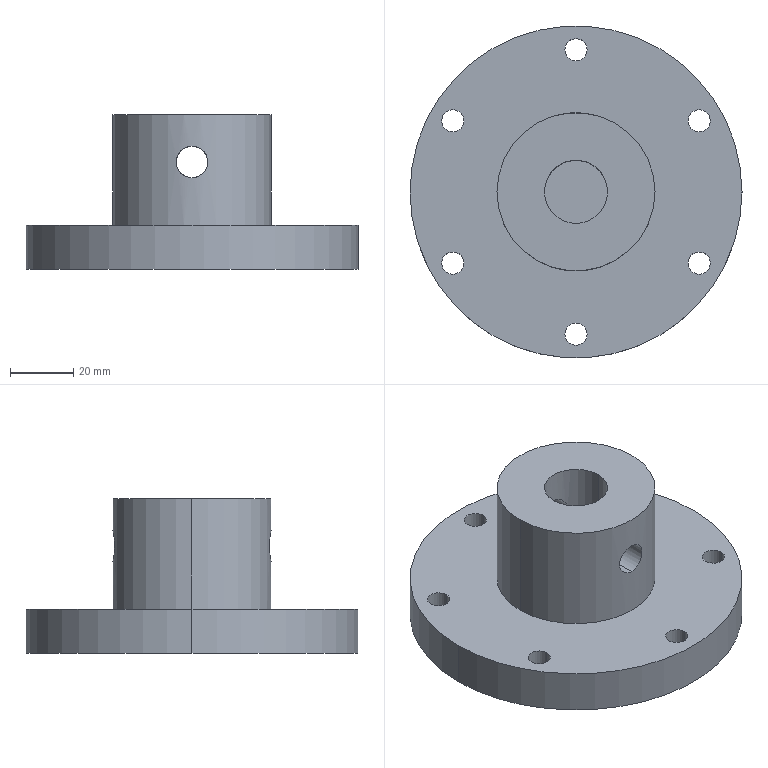Part | SolidWorks | features ICE 2, Extrusion 1 | 1 solid | 26 faces | box 105 x 105 x 49 mm | volume 173332 mm3 | cylinder 22 | plane 4 | commonest cylinder face diameters 7 x12 10 x4 20 x2 50 x2 105 x2
STEP:
#1=CARTESIAN_POINT('',(0.,-25.,29.));
#2=VERTEX_POINT('',#1);
#3=CARTESIAN_POINT('',(0.,-25.,39.));
#4=VERTEX_POINT('',#3);
#5=CARTESIAN_POINT('',(0.,-25.,29.));
#6=CARTESIAN_POINT('',(-0.3267,-25.,29.));
#7=CARTESIAN_POINT('',(-0.652,-24.994,29.032));
#8=CARTESIAN_POINT('',(-1.3,-24.968,29.161));
#9=CARTESIAN_POINT('',(-1.614,-24.95,29.256));
#10=CARTESIAN_POINT('',(-2.065,-24.915,29.444));
#11=CARTESIAN_POINT('',(-2.213,-24.902,29.513));
#12=CARTESIAN_POINT('',(-2.502,-24.875,29.668));
#13=CARTESIAN_POINT('',(-2.644,-24.86,29.753));
#14=CARTESIAN_POINT('',(-3.052,-24.815,30.026));
#15=CARTESIAN_POINT('',(-3.303,-24.782,30.232));
#16=CARTESIAN_POINT('',(-3.764,-24.716,30.693));
#17=CARTESIAN_POINT('',(-3.975,-24.683,30.949));
#18=CARTESIAN_POINT('',(-4.337,-24.622,31.49));
#19=CARTESIAN_POINT('',(-4.491,-24.594,31.777));
#20=CARTESIAN_POINT('',(-4.743,-24.546,32.384));
#21=CARTESIAN_POINT('',(-4.839,-24.527,32.7));
#22=CARTESIAN_POINT('',(-4.967,-24.502,33.34));
#23=CARTESIAN_POINT('',(-5.,-24.495,33.667));
#24=CARTESIAN_POINT('',(-5.,-24.495,34.328));
#25=CARTESIAN_POINT('',(-4.968,-24.502,34.653));
#26=CARTESIAN_POINT('',(-4.841,-24.527,35.294));
#27=CARTESIAN_POINT('',(-4.744,-24.546,35.612));
#28=CARTESIAN_POINT('',(-4.494,-24.593,36.216));
#29=CARTESIAN_POINT('',(-4.341,-24.621,36.503));
#30=CARTESIAN_POINT('',(-4.068,-24.667,36.912));
#31=CARTESIAN_POINT('',(-3.97,-24.683,37.045));
#32=CARTESIAN_POINT('',(-3.762,-24.716,37.298));
#33=CARTESIAN_POINT('',(-3.653,-24.732,37.418));
#34=CARTESIAN_POINT('',(-3.308,-24.781,37.763));
#35=CARTESIAN_POINT('',(-3.057,-24.814,37.971));
#36=CARTESIAN_POINT('',(-2.509,-24.875,38.337));
#37=CARTESIAN_POINT('',(-2.222,-24.903,38.491));
#38=CARTESIAN_POINT('',(-1.62,-24.949,38.741));
#39=CARTESIAN_POINT('',(-1.303,-24.968,38.838));
#40=CARTESIAN_POINT('',(-0.658,-24.993,38.967));
#41=CARTESIAN_POINT('',(-0.3312,-25.,39.));
#42=CARTESIAN_POINT('',(0.,-25.,39.));
#43=B_SPLINE_CURVE_WITH_KNOTS('',3,(#5,#6,#7,#8,#9,#10,#11,#12,#13,#14,#15,#16,#17,#18,#19,#20,#21,#22,#23,#24,#25,#26,#27,#28,#29,#30,#31,#32,#33,#34,#35,#36,#37,#38,#39,#40,#41,#42),.UNSPECIFIED.,.F.,.F.,(4,2,2,2,2,2,2,2,2,2,2,2,2,2,2,2,2,2,4),(0.01567,0.01665,0.01763,0.01812,0.01861,0.01959,0.02057,0.02155,0.02253,0.02351,0.02449,0.02546,0.02644,0.02693,0.02742,0.0284,0.02938,0.03036,0.03134),.UNSPECIFIED.);
#44=EDGE_CURVE('',#2,#4,#43,.T.);
#45=ORIENTED_EDGE('',*,*,#44,.F.);
#46=CARTESIAN_POINT('',(0.,-10.,29.));
#47=VERTEX_POINT('',#46);
#48=CARTESIAN_POINT('',(0.,-52.5,29.));
#49=DIRECTION('',(0.,1.,0.));
#50=VECTOR('',#49,1000.);
#51=LINE('',#48,#50);
#52=EDGE_CURVE('',#2,#47,#51,.T.);
#53=ORIENTED_EDGE('',*,*,#52,.T.);
#54=CARTESIAN_POINT('',(0.,-10.,39.));
#55=VERTEX_POINT('',#54);
#56=CARTESIAN_POINT('',(0.,-10.,29.));
#57=CARTESIAN_POINT('',(-0.3314,-10.,29.));
#58=CARTESIAN_POINT('',(-0.6687,-9.983,29.034));
#59=CARTESIAN_POINT('',(-1.317,-9.918,29.165));
#60=CARTESIAN_POINT('',(-1.631,-9.871,29.262));
#61=CARTESIAN_POINT('',(-2.24,-9.751,29.518));
#62=CARTESIAN_POINT('',(-2.526,-9.68,29.673));
#63=CARTESIAN_POINT('',(-3.061,-9.524,30.034));
#64=CARTESIAN_POINT('',(-3.314,-9.438,30.242));
#65=CARTESIAN_POINT('',(-3.767,-9.266,30.697));
#66=CARTESIAN_POINT('',(-3.971,-9.18,30.944));
#67=CARTESIAN_POINT('',(-4.331,-9.016,31.48));
#68=CARTESIAN_POINT('',(-4.487,-8.938,31.769));
#69=CARTESIAN_POINT('',(-4.737,-8.808,32.367));
#70=CARTESIAN_POINT('',(-4.834,-8.754,32.679));
#71=CARTESIAN_POINT('',(-4.933,-8.699,33.168));
#72=CARTESIAN_POINT('',(-4.958,-8.684,33.334));
#73=CARTESIAN_POINT('',(-4.991,-8.665,33.664));
#74=CARTESIAN_POINT('',(-5.008,-8.656,33.994));
#75=CARTESIAN_POINT('',(-4.992,-8.665,34.325));
#76=CARTESIAN_POINT('',(-4.959,-8.684,34.657));
#77=CARTESIAN_POINT('',(-4.935,-8.698,34.823));
#78=CARTESIAN_POINT('',(-4.836,-8.753,35.311));
#79=CARTESIAN_POINT('',(-4.74,-8.806,35.625));
#80=CARTESIAN_POINT('',(-4.487,-8.938,36.23));
#81=CARTESIAN_POINT('',(-4.332,-9.015,36.518));
#82=CARTESIAN_POINT('',(-3.973,-9.179,37.053));
#83=CARTESIAN_POINT('',(-3.767,-9.267,37.304));
#84=CARTESIAN_POINT('',(-3.311,-9.439,37.761));
#85=CARTESIAN_POINT('',(-3.064,-9.523,37.965));
#86=CARTESIAN_POINT('',(-2.528,-9.679,38.326));
#87=CARTESIAN_POINT('',(-2.237,-9.751,38.483));
#88=CARTESIAN_POINT('',(-1.635,-9.87,38.736));
#89=CARTESIAN_POINT('',(-1.323,-9.918,38.833));
#90=CARTESIAN_POINT('',(-0.6735,-9.983,38.965));
#91=CARTESIAN_POINT('',(-0.3359,-10.,39.));
#92=CARTESIAN_POINT('',(0.,-10.,39.));
#93=B_SPLINE_CURVE_WITH_KNOTS('',3,(#56,#57,#58,#59,#60,#61,#62,#63,#64,#65,#66,#67,#68,#69,#70,#71,#72,#73,#74,#75,#76,#77,#78,#79,#80,#81,#82,#83,#84,#85,#86,#87,#88,#89,#90,#91,#92),.UNSPECIFIED.,.F.,.F.,(4,2,2,2,2,2,2,2,2,1,2,2,2,2,2,2,2,2,4),(0.0159,0.0169,0.01789,0.01888,0.01987,0.02087,0.02186,0.02285,0.02335,0.02384,0.02434,0.02484,0.02583,0.02682,0.02781,0.02881,0.0298,0.03079,0.03178),.UNSPECIFIED.);
#94=EDGE_CURVE('',#47,#55,#93,.T.);
#95=ORIENTED_EDGE('',*,*,#94,.T.);
#96=CARTESIAN_POINT('',(0.,-52.5,39.));
#97=DIRECTION('',(0.,1.,0.));
#98=VECTOR('',#97,1000.);
#99=LINE('',#96,#98);
#100=EDGE_CURVE('',#4,#55,#99,.T.);
#101=ORIENTED_EDGE('',*,*,#100,.F.);
#102=EDGE_LOOP('',(#45,#53,#95,#101));
#103=FACE_OUTER_BOUND('',#102,.T.);
#104=CARTESIAN_POINT('',(0.,-52.5,34.));
#105=DIRECTION('',(0.,1.,0.));
#106=DIRECTION('',(0.,0.,1.));
#107=AXIS2_PLACEMENT_3D('',#104,#105,#106);
#108=CYLINDRICAL_SURFACE('',#107,5.);
#109=ADVANCED_FACE('',(#103),#108,.F.);
#110=CARTESIAN_POINT('',(0.,10.,39.));
#111=VERTEX_POINT('',#110);
#112=CARTESIAN_POINT('',(0.,10.,29.));
#113=VERTEX_POINT('',#112);
#114=CARTESIAN_POINT('',(0.,10.,39.));
#115=CARTESIAN_POINT('',(-0.3365,10.,39.));
#116=CARTESIAN_POINT('',(-0.6663,9.983,38.966));
#117=CARTESIAN_POINT('',(-1.314,9.919,38.836));
#118=CARTESIAN_POINT('',(-1.634,9.87,38.737));
#119=CARTESIAN_POINT('',(-2.238,9.751,38.483));
#120=CARTESIAN_POINT('',(-2.523,9.68,38.329));
#121=CARTESIAN_POINT('',(-3.063,9.524,37.965));
#122=CARTESIAN_POINT('',(-3.313,9.438,37.758));
#123=CARTESIAN_POINT('',(-3.766,9.267,37.305));
#124=CARTESIAN_POINT('',(-3.972,9.179,37.054));
#125=CARTESIAN_POINT('',(-4.333,9.015,36.516));
#126=CARTESIAN_POINT('',(-4.486,8.939,36.232));
#127=CARTESIAN_POINT('',(-4.674,8.841,35.783));
#128=CARTESIAN_POINT('',(-4.73,8.811,35.629));
#129=CARTESIAN_POINT('',(-4.827,8.758,35.313));
#130=CARTESIAN_POINT('',(-4.868,8.735,35.152));
#131=CARTESIAN_POINT('',(-4.966,8.68,34.666));
#132=CARTESIAN_POINT('',(-5.,8.66,34.338));
#133=CARTESIAN_POINT('',(-5.,8.66,33.838));
#134=CARTESIAN_POINT('',(-4.992,8.665,33.67));
#135=CARTESIAN_POINT('',(-4.959,8.684,33.337));
#136=CARTESIAN_POINT('',(-4.934,8.698,33.173));
#137=CARTESIAN_POINT('',(-4.836,8.753,32.688));
#138=CARTESIAN_POINT('',(-4.738,8.807,32.37));
#139=CARTESIAN_POINT('',(-4.485,8.939,31.765));
#140=CARTESIAN_POINT('',(-4.331,9.016,31.48));
#141=CARTESIAN_POINT('',(-3.97,9.18,30.943));
#142=CARTESIAN_POINT('',(-3.763,9.268,30.692));
#143=CARTESIAN_POINT('',(-3.309,9.44,30.238));
#144=CARTESIAN_POINT('',(-3.061,9.524,30.033));
#145=CARTESIAN_POINT('',(-2.52,9.681,29.669));
#146=CARTESIAN_POINT('',(-2.233,9.752,29.514));
#147=CARTESIAN_POINT('',(-1.783,9.841,29.326));
#148=CARTESIAN_POINT('',(-1.629,9.868,29.27));
#149=CARTESIAN_POINT('',(-1.314,9.915,29.173));
#150=CARTESIAN_POINT('',(-1.152,9.935,29.132));
#151=CARTESIAN_POINT('',(-0.6614,9.984,29.033));
#152=CARTESIAN_POINT('',(-0.332,10.,29.));
#153=CARTESIAN_POINT('',(0.,10.,29.));
#154=B_SPLINE_CURVE_WITH_KNOTS('',3,(#114,#115,#116,#117,#118,#119,#120,#121,#122,#123,#124,#125,#126,#127,#128,#129,#130,#131,#132,#133,#134,#135,#136,#137,#138,#139,#140,#141,#142,#143,#144,#145,#146,#147,#148,#149,#150,#151,#152,#153),.UNSPECIFIED.,.F.,.F.,(4,2,2,2,2,2,2,2,2,2,2,2,2,2,2,2,2,2,2,4),(0.,0.0009941,0.001988,0.002982,0.003976,0.00497,0.005964,0.006461,0.006958,0.007952,0.008449,0.008947,0.009941,0.01093,0.01193,0.01292,0.01392,0.01441,0.01491,0.0159),.UNSPECIFIED.);
#155=EDGE_CURVE('',#111,#113,#154,.T.);
#156=ORIENTED_EDGE('',*,*,#155,.T.);
#157=CARTESIAN_POINT('',(0.,25.,29.));
#158=VERTEX_POINT('',#157);
#159=CARTESIAN_POINT('',(0.,-52.5,29.));
#160=DIRECTION('',(0.,1.,0.));
#161=VECTOR('',#160,1000.);
#162=LINE('',#159,#161);
#163=EDGE_CURVE('',#113,#158,#162,.T.);
#164=ORIENTED_EDGE('',*,*,#163,.T.);
#165=CARTESIAN_POINT('',(0.,25.,39.));
#166=VERTEX_POINT('',#165);
#167=CARTESIAN_POINT('',(0.,25.,39.));
#168=CARTESIAN_POINT('',(-0.3313,25.,39.));
#169=CARTESIAN_POINT('',(-0.6568,24.993,38.967));
#170=CARTESIAN_POINT('',(-1.297,24.968,38.84));
#171=CARTESIAN_POINT('',(-1.615,24.95,38.743));
#172=CARTESIAN_POINT('',(-2.22,24.903,38.492));
#173=CARTESIAN_POINT('',(-2.507,24.875,38.338));
#174=CARTESIAN_POINT('',(-3.05,24.815,37.975));
#175=CARTESIAN_POINT('',(-3.306,24.781,37.765));
#176=CARTESIAN_POINT('',(-3.766,24.716,37.305));
#177=CARTESIAN_POINT('',(-3.973,24.683,37.053));
#178=CARTESIAN_POINT('',(-4.339,24.621,36.507));
#179=CARTESIAN_POINT('',(-4.493,24.593,36.217));
#180=CARTESIAN_POINT('',(-4.743,24.546,35.616));
#181=CARTESIAN_POINT('',(-4.839,24.527,35.3));
#182=CARTESIAN_POINT('',(-4.968,24.502,34.654));
#183=CARTESIAN_POINT('',(-5.,24.495,34.329));
#184=CARTESIAN_POINT('',(-5.,24.495,33.675));
#185=CARTESIAN_POINT('',(-4.967,24.502,33.343));
#186=CARTESIAN_POINT('',(-4.839,24.527,32.701));
#187=CARTESIAN_POINT('',(-4.745,24.546,32.389));
#188=CARTESIAN_POINT('',(-4.556,24.581,31.934));
#189=CARTESIAN_POINT('',(-4.485,24.595,31.784));
#190=CARTESIAN_POINT('',(-4.33,24.622,31.495));
#191=CARTESIAN_POINT('',(-4.247,24.637,31.356));
#192=CARTESIAN_POINT('',(-3.975,24.683,30.95));
#193=CARTESIAN_POINT('',(-3.768,24.716,30.697));
#194=CARTESIAN_POINT('',(-3.303,24.782,30.232));
#195=CARTESIAN_POINT('',(-3.051,24.815,30.026));
#196=CARTESIAN_POINT('',(-2.51,24.875,29.664));
#197=CARTESIAN_POINT('',(-2.218,24.903,29.507));
#198=CARTESIAN_POINT('',(-1.613,24.95,29.256));
#199=CARTESIAN_POINT('',(-1.301,24.968,29.161));
#200=CARTESIAN_POINT('',(-0.6587,24.993,29.033));
#201=CARTESIAN_POINT('',(-0.3268,25.,29.));
#202=CARTESIAN_POINT('',(0.,25.,29.));
#203=B_SPLINE_CURVE_WITH_KNOTS('',3,(#167,#168,#169,#170,#171,#172,#173,#174,#175,#176,#177,#178,#179,#180,#181,#182,#183,#184,#185,#186,#187,#188,#189,#190,#191,#192,#193,#194,#195,#196,#197,#198,#199,#200,#201,#202),.UNSPECIFIED.,.F.,.F.,(4,2,2,2,2,2,2,2,2,2,2,2,2,2,2,2,2,4),(0.,0.0009795,0.001959,0.002938,0.003918,0.004897,0.005877,0.006856,0.007836,0.008815,0.009795,0.01028,0.01077,0.01175,0.01273,0.01371,0.01469,0.01567),.UNSPECIFIED.);
#204=EDGE_CURVE('',#166,#158,#203,.T.);
#205=ORIENTED_EDGE('',*,*,#204,.F.);
#206=CARTESIAN_POINT('',(0.,-52.5,39.));
#207=DIRECTION('',(0.,1.,0.));
#208=VECTOR('',#207,1000.);
#209=LINE('',#206,#208);
#210=EDGE_CURVE('',#111,#166,#209,.T.);
#211=ORIENTED_EDGE('',*,*,#210,.F.);
#212=EDGE_LOOP('',(#156,#164,#205,#211));
#213=FACE_OUTER_BOUND('',#212,.T.);
#214=CARTESIAN_POINT('',(0.,-52.5,34.));
#215=DIRECTION('',(0.,1.,0.));
#216=DIRECTION('',(0.,0.,1.));
#217=AXIS2_PLACEMENT_3D('',#214,#215,#216);
#218=CYLINDRICAL_SURFACE('',#217,5.);
#219=ADVANCED_FACE('',(#213),#218,.F.);
#220=CARTESIAN_POINT('',(0.,-10.,39.));
#221=CARTESIAN_POINT('',(0.3365,-10.,39.));
#222=CARTESIAN_POINT('',(0.6663,-9.983,38.966));
#223=CARTESIAN_POINT('',(1.314,-9.919,38.836));
#224=CARTESIAN_POINT('',(1.634,-9.87,38.737));
#225=CARTESIAN_POINT('',(2.238,-9.751,38.483));
#226=CARTESIAN_POINT('',(2.523,-9.68,38.329));
#227=CARTESIAN_POINT('',(3.063,-9.524,37.965));
#228=CARTESIAN_POINT('',(3.313,-9.438,37.758));
#229=CARTESIAN_POINT('',(3.766,-9.267,37.305));
#230=CARTESIAN_POINT('',(3.972,-9.179,37.054));
#231=CARTESIAN_POINT('',(4.333,-9.015,36.516));
#232=CARTESIAN_POINT('',(4.486,-8.939,36.232));
#233=CARTESIAN_POINT('',(4.674,-8.841,35.783));
#234=CARTESIAN_POINT('',(4.73,-8.811,35.629));
#235=CARTESIAN_POINT('',(4.827,-8.758,35.313));
#236=CARTESIAN_POINT('',(4.868,-8.735,35.152));
#237=CARTESIAN_POINT('',(4.966,-8.68,34.666));
#238=CARTESIAN_POINT('',(5.,-8.66,34.338));
#239=CARTESIAN_POINT('',(5.,-8.66,33.838));
#240=CARTESIAN_POINT('',(4.992,-8.665,33.67));
#241=CARTESIAN_POINT('',(4.959,-8.684,33.337));
#242=CARTESIAN_POINT('',(4.934,-8.698,33.173));
#243=CARTESIAN_POINT('',(4.836,-8.753,32.688));
#244=CARTESIAN_POINT('',(4.738,-8.807,32.37));
#245=CARTESIAN_POINT('',(4.485,-8.939,31.765));
#246=CARTESIAN_POINT('',(4.331,-9.016,31.48));
#247=CARTESIAN_POINT('',(3.97,-9.18,30.943));
#248=CARTESIAN_POINT('',(3.763,-9.268,30.692));
#249=CARTESIAN_POINT('',(3.309,-9.44,30.238));
#250=CARTESIAN_POINT('',(3.061,-9.524,30.033));
#251=CARTESIAN_POINT('',(2.52,-9.681,29.669));
#252=CARTESIAN_POINT('',(2.233,-9.752,29.514));
#253=CARTESIAN_POINT('',(1.783,-9.841,29.326));
#254=CARTESIAN_POINT('',(1.629,-9.868,29.27));
#255=CARTESIAN_POINT('',(1.314,-9.915,29.173));
#256=CARTESIAN_POINT('',(1.152,-9.935,29.132));
#257=CARTESIAN_POINT('',(0.6614,-9.984,29.033));
#258=CARTESIAN_POINT('',(0.332,-10.,29.));
#259=CARTESIAN_POINT('',(0.,-10.,29.));
#260=B_SPLINE_CURVE_WITH_KNOTS('',3,(#220,#221,#222,#223,#224,#225,#226,#227,#228,#229,#230,#231,#232,#233,#234,#235,#236,#237,#238,#239,#240,#241,#242,#243,#244,#245,#246,#247,#248,#249,#250,#251,#252,#253,#254,#255,#256,#257,#258,#259),.UNSPECIFIED.,.F.,.F.,(4,2,2,2,2,2,2,2,2,2,2,2,2,2,2,2,2,2,2,4),(0.,0.0009941,0.001988,0.002982,0.003976,0.00497,0.005964,0.006461,0.006958,0.007952,0.008449,0.008947,0.009941,0.01093,0.01193,0.01292,0.01392,0.01441,0.01491,0.0159),.UNSPECIFIED.);
#261=EDGE_CURVE('',#55,#47,#260,.T.);
#262=ORIENTED_EDGE('',*,*,#261,.F.);
#263=ORIENTED_EDGE('',*,*,#94,.F.);
#264=EDGE_LOOP('',(#262,#263));
#265=FACE_BOUND('',#264,.T.);
#266=CARTESIAN_POINT('',(-10.,0.,49.));
#267=VERTEX_POINT('',#266);
#268=CARTESIAN_POINT('',(10.,0.,49.));
#269=VERTEX_POINT('',#268);
#270=CARTESIAN_POINT('',(0.,0.,49.));
#271=DIRECTION('',(0.,0.,1.));
#272=DIRECTION('',(1.,0.,0.));
#273=AXIS2_PLACEMENT_3D('',#270,#271,#272);
#274=CIRCLE('',#273,10.);
#275=EDGE_CURVE('',#267,#269,#274,.T.);
#276=ORIENTED_EDGE('',*,*,#275,.T.);
#277=CARTESIAN_POINT('',(10.,0.,14.));
#278=VERTEX_POINT('',#277);
#279=CARTESIAN_POINT('',(10.,0.,49.));
#280=DIRECTION('',(0.,0.,-1.));
#281=VECTOR('',#280,1000.);
#282=LINE('',#279,#281);
#283=EDGE_CURVE('',#269,#278,#282,.T.);
#284=ORIENTED_EDGE('',*,*,#283,.T.);
#285=CARTESIAN_POINT('',(-10.,0.,14.));
#286=VERTEX_POINT('',#285);
#287=CARTESIAN_POINT('',(0.,0.,14.));
#288=DIRECTION('',(0.,0.,-1.));
#289=DIRECTION('',(1.,0.,0.));
#290=AXIS2_PLACEMENT_3D('',#287,#288,#289);
#291=CIRCLE('',#290,10.);
#292=EDGE_CURVE('',#278,#286,#291,.T.);
#293=ORIENTED_EDGE('',*,*,#292,.T.);
#294=CARTESIAN_POINT('',(-10.,0.,49.));
#295=DIRECTION('',(0.,0.,-1.));
#296=VECTOR('',#295,1000.);
#297=LINE('',#294,#296);
#298=EDGE_CURVE('',#267,#286,#297,.T.);
#299=ORIENTED_EDGE('',*,*,#298,.F.);
#300=EDGE_LOOP('',(#276,#284,#293,#299));
#301=FACE_OUTER_BOUND('',#300,.T.);
#302=CARTESIAN_POINT('',(0.,0.,49.));
#303=DIRECTION('',(0.,0.,-1.));
#304=DIRECTION('',(-1.,0.,0.));
#305=AXIS2_PLACEMENT_3D('',#302,#303,#304);
#306=CYLINDRICAL_SURFACE('',#305,10.);
#307=ADVANCED_FACE('',(#265,#301),#306,.F.);
#308=ORIENTED_EDGE('',*,*,#204,.T.);
#309=CARTESIAN_POINT('',(0.,25.,29.));
#310=CARTESIAN_POINT('',(0.3267,25.,29.));
#311=CARTESIAN_POINT('',(0.652,24.994,29.032));
#312=CARTESIAN_POINT('',(1.3,24.968,29.161));
#313=CARTESIAN_POINT('',(1.614,24.95,29.256));
#314=CARTESIAN_POINT('',(2.065,24.915,29.444));
#315=CARTESIAN_POINT('',(2.213,24.902,29.513));
#316=CARTESIAN_POINT('',(2.502,24.875,29.668));
#317=CARTESIAN_POINT('',(2.644,24.86,29.753));
#318=CARTESIAN_POINT('',(3.052,24.815,30.026));
#319=CARTESIAN_POINT('',(3.303,24.782,30.232));
#320=CARTESIAN_POINT('',(3.764,24.716,30.693));
#321=CARTESIAN_POINT('',(3.975,24.683,30.949));
#322=CARTESIAN_POINT('',(4.337,24.622,31.49));
#323=CARTESIAN_POINT('',(4.491,24.594,31.777));
#324=CARTESIAN_POINT('',(4.743,24.546,32.384));
#325=CARTESIAN_POINT('',(4.839,24.527,32.7));
#326=CARTESIAN_POINT('',(4.967,24.502,33.34));
#327=CARTESIAN_POINT('',(5.,24.495,33.667));
#328=CARTESIAN_POINT('',(5.,24.495,34.328));
#329=CARTESIAN_POINT('',(4.968,24.502,34.653));
#330=CARTESIAN_POINT('',(4.841,24.527,35.294));
#331=CARTESIAN_POINT('',(4.744,24.546,35.612));
#332=CARTESIAN_POINT('',(4.494,24.593,36.216));
#333=CARTESIAN_POINT('',(4.341,24.621,36.503));
#334=CARTESIAN_POINT('',(4.068,24.667,36.912));
#335=CARTESIAN_POINT('',(3.97,24.683,37.045));
#336=CARTESIAN_POINT('',(3.762,24.716,37.298));
#337=CARTESIAN_POINT('',(3.653,24.732,37.418));
#338=CARTESIAN_POINT('',(3.308,24.781,37.763));
#339=CARTESIAN_POINT('',(3.057,24.814,37.971));
#340=CARTESIAN_POINT('',(2.509,24.875,38.337));
#341=CARTESIAN_POINT('',(2.222,24.903,38.491));
#342=CARTESIAN_POINT('',(1.62,24.949,38.741));
#343=CARTESIAN_POINT('',(1.303,24.968,38.838));
#344=CARTESIAN_POINT('',(0.658,24.993,38.967));
#345=CARTESIAN_POINT('',(0.3312,25.,39.));
#346=CARTESIAN_POINT('',(0.,25.,39.));
#347=B_SPLINE_CURVE_WITH_KNOTS('',3,(#309,#310,#311,#312,#313,#314,#315,#316,#317,#318,#319,#320,#321,#322,#323,#324,#325,#326,#327,#328,#329,#330,#331,#332,#333,#334,#335,#336,#337,#338,#339,#340,#341,#342,#343,#344,#345,#346),.UNSPECIFIED.,.F.,.F.,(4,2,2,2,2,2,2,2,2,2,2,2,2,2,2,2,2,2,4),(0.01567,0.01665,0.01763,0.01812,0.01861,0.01959,0.02057,0.02155,0.02253,0.02351,0.02449,0.02546,0.02644,0.02693,0.02742,0.0284,0.02938,0.03036,0.03134),.UNSPECIFIED.);
#348=EDGE_CURVE('',#158,#166,#347,.T.);
#349=ORIENTED_EDGE('',*,*,#348,.T.);
#350=EDGE_LOOP('',(#308,#349));
#351=FACE_BOUND('',#350,.T.);
#352=CARTESIAN_POINT('',(25.,0.,49.));
#353=VERTEX_POINT('',#352);
#354=CARTESIAN_POINT('',(-25.,0.,49.));
#355=VERTEX_POINT('',#354);
#356=CARTESIAN_POINT('',(0.,0.,49.));
#357=DIRECTION('',(0.,0.,1.));
#358=DIRECTION('',(1.,0.,0.));
#359=AXIS2_PLACEMENT_3D('',#356,#357,#358);
#360=CIRCLE('',#359,25.);
#361=EDGE_CURVE('',#353,#355,#360,.T.);
#362=ORIENTED_EDGE('',*,*,#361,.F.);
#363=CARTESIAN_POINT('',(25.,0.,14.));
#364=VERTEX_POINT('',#363);
#365=CARTESIAN_POINT('',(25.,0.,49.));
#366=DIRECTION('',(0.,0.,-1.));
#367=VECTOR('',#366,1000.);
#368=LINE('',#365,#367);
#369=EDGE_CURVE('',#353,#364,#368,.T.);
#370=ORIENTED_EDGE('',*,*,#369,.T.);
#371=CARTESIAN_POINT('',(-25.,0.,14.));
#372=VERTEX_POINT('',#371);
#373=CARTESIAN_POINT('',(0.,0.,14.));
#374=DIRECTION('',(0.,0.,1.));
#375=DIRECTION('',(1.,0.,0.));
#376=AXIS2_PLACEMENT_3D('',#373,#374,#375);
#377=CIRCLE('',#376,25.);
#378=EDGE_CURVE('',#364,#372,#377,.T.);
#379=ORIENTED_EDGE('',*,*,#378,.T.);
#380=CARTESIAN_POINT('',(-25.,0.,49.));
#381=DIRECTION('',(0.,0.,-1.));
#382=VECTOR('',#381,1000.);
#383=LINE('',#380,#382);
#384=EDGE_CURVE('',#355,#372,#383,.T.);
#385=ORIENTED_EDGE('',*,*,#384,.F.);
#386=EDGE_LOOP('',(#362,#370,#379,#385));
#387=FACE_OUTER_BOUND('',#386,.T.);
#388=CARTESIAN_POINT('',(0.,0.,49.));
#389=DIRECTION('',(0.,0.,-1.));
#390=DIRECTION('',(-1.,0.,0.));
#391=AXIS2_PLACEMENT_3D('',#388,#389,#390);
#392=CYLINDRICAL_SURFACE('',#391,25.);
#393=ADVANCED_FACE('',(#351,#387),#392,.T.);
#394=CARTESIAN_POINT('',(-42.471,22.5,14.));
#395=VERTEX_POINT('',#394);
#396=CARTESIAN_POINT('',(-35.471,22.5,14.));
#397=VERTEX_POINT('',#396);
#398=CARTESIAN_POINT('',(-38.971,22.5,14.));
#399=DIRECTION('',(0.,0.,1.));
#400=DIRECTION('',(1.,0.,0.));
#401=AXIS2_PLACEMENT_3D('',#398,#399,#400);
#402=CIRCLE('',#401,3.5);
#403=EDGE_CURVE('',#395,#397,#402,.T.);
#404=ORIENTED_EDGE('',*,*,#403,.T.);
#405=CARTESIAN_POINT('',(-35.471,22.5,0.));
#406=VERTEX_POINT('',#405);
#407=CARTESIAN_POINT('',(-35.471,22.5,14.));
#408=DIRECTION('',(0.,0.,-1.));
#409=VECTOR('',#408,1000.);
#410=LINE('',#407,#409);
#411=EDGE_CURVE('',#397,#406,#410,.T.);
#412=ORIENTED_EDGE('',*,*,#411,.T.);
#413=CARTESIAN_POINT('',(-42.471,22.5,0.));
#414=VERTEX_POINT('',#413);
#415=CARTESIAN_POINT('',(-38.971,22.5,0.));
#416=DIRECTION('',(0.,0.,1.));
#417=DIRECTION('',(1.,0.,0.));
#418=AXIS2_PLACEMENT_3D('',#415,#416,#417);
#419=CIRCLE('',#418,3.5);
#420=EDGE_CURVE('',#414,#406,#419,.T.);
#421=ORIENTED_EDGE('',*,*,#420,.F.);
#422=CARTESIAN_POINT('',(-42.471,22.5,14.));
#423=DIRECTION('',(0.,0.,-1.));
#424=VECTOR('',#423,1000.);
#425=LINE('',#422,#424);
#426=EDGE_CURVE('',#395,#414,#425,.T.);
#427=ORIENTED_EDGE('',*,*,#426,.F.);
#428=EDGE_LOOP('',(#404,#412,#421,#427));
#429=FACE_OUTER_BOUND('',#428,.T.);
#430=CARTESIAN_POINT('',(-38.971,22.5,14.));
#431=DIRECTION('',(0.,0.,-1.));
#432=DIRECTION('',(-1.,0.,0.));
#433=AXIS2_PLACEMENT_3D('',#430,#431,#432);
#434=CYLINDRICAL_SURFACE('',#433,3.5);
#435=ADVANCED_FACE('',(#429),#434,.F.);
#436=CARTESIAN_POINT('',(-42.471,-22.5,14.));
#437=VERTEX_POINT('',#436);
#438=CARTESIAN_POINT('',(-35.471,-22.5,14.));
#439=VERTEX_POINT('',#438);
#440=CARTESIAN_POINT('',(-38.971,-22.5,14.));
#441=DIRECTION('',(0.,0.,1.));
#442=DIRECTION('',(1.,0.,0.));
#443=AXIS2_PLACEMENT_3D('',#440,#441,#442);
#444=CIRCLE('',#443,3.5);
#445=EDGE_CURVE('',#437,#439,#444,.T.);
#446=ORIENTED_EDGE('',*,*,#445,.T.);
#447=CARTESIAN_POINT('',(-35.471,-22.5,0.));
#448=VERTEX_POINT('',#447);
#449=CARTESIAN_POINT('',(-35.471,-22.5,14.));
#450=DIRECTION('',(0.,0.,-1.));
#451=VECTOR('',#450,1000.);
#452=LINE('',#449,#451);
#453=EDGE_CURVE('',#439,#448,#452,.T.);
#454=ORIENTED_EDGE('',*,*,#453,.T.);
#455=CARTESIAN_POINT('',(-42.471,-22.5,0.));
#456=VERTEX_POINT('',#455);
#457=CARTESIAN_POINT('',(-38.971,-22.5,0.));
#458=DIRECTION('',(0.,0.,1.));
#459=DIRECTION('',(1.,0.,0.));
#460=AXIS2_PLACEMENT_3D('',#457,#458,#459);
#461=CIRCLE('',#460,3.5);
#462=EDGE_CURVE('',#456,#448,#461,.T.);
#463=ORIENTED_EDGE('',*,*,#462,.F.);
#464=CARTESIAN_POINT('',(-42.471,-22.5,14.));
#465=DIRECTION('',(0.,0.,-1.));
#466=VECTOR('',#465,1000.);
#467=LINE('',#464,#466);
#468=EDGE_CURVE('',#437,#456,#467,.T.);
#469=ORIENTED_EDGE('',*,*,#468,.F.);
#470=EDGE_LOOP('',(#446,#454,#463,#469));
#471=FACE_OUTER_BOUND('',#470,.T.);
#472=CARTESIAN_POINT('',(-38.971,-22.5,14.));
#473=DIRECTION('',(0.,0.,-1.));
#474=DIRECTION('',(-1.,0.,0.));
#475=AXIS2_PLACEMENT_3D('',#472,#473,#474);
#476=CYLINDRICAL_SURFACE('',#475,3.5);
#477=ADVANCED_FACE('',(#471),#476,.F.);
#478=CARTESIAN_POINT('',(-3.5,-45.,14.));
#479=VERTEX_POINT('',#478);
#480=CARTESIAN_POINT('',(3.5,-45.,14.));
#481=VERTEX_POINT('',#480);
#482=CARTESIAN_POINT('',(0.,-45.,14.));
#483=DIRECTION('',(0.,0.,1.));
#484=DIRECTION('',(1.,0.,0.));
#485=AXIS2_PLACEMENT_3D('',#482,#483,#484);
#486=CIRCLE('',#485,3.5);
#487=EDGE_CURVE('',#479,#481,#486,.T.);
#488=ORIENTED_EDGE('',*,*,#487,.T.);
#489=CARTESIAN_POINT('',(3.5,-45.,0.));
#490=VERTEX_POINT('',#489);
#491=CARTESIAN_POINT('',(3.5,-45.,14.));
#492=DIRECTION('',(0.,0.,-1.));
#493=VECTOR('',#492,1000.);
#494=LINE('',#491,#493);
#495=EDGE_CURVE('',#481,#490,#494,.T.);
#496=ORIENTED_EDGE('',*,*,#495,.T.);
#497=CARTESIAN_POINT('',(-3.5,-45.,0.));
#498=VERTEX_POINT('',#497);
#499=CARTESIAN_POINT('',(0.,-45.,0.));
#500=DIRECTION('',(0.,0.,1.));
#501=DIRECTION('',(1.,0.,0.));
#502=AXIS2_PLACEMENT_3D('',#499,#500,#501);
#503=CIRCLE('',#502,3.5);
#504=EDGE_CURVE('',#498,#490,#503,.T.);
#505=ORIENTED_EDGE('',*,*,#504,.F.);
#506=CARTESIAN_POINT('',(-3.5,-45.,14.));
#507=DIRECTION('',(0.,0.,-1.));
#508=VECTOR('',#507,1000.);
#509=LINE('',#506,#508);
#510=EDGE_CURVE('',#479,#498,#509,.T.);
#511=ORIENTED_EDGE('',*,*,#510,.F.);
#512=EDGE_LOOP('',(#488,#496,#505,#511));
#513=FACE_OUTER_BOUND('',#512,.T.);
#514=CARTESIAN_POINT('',(0.,-45.,14.));
#515=DIRECTION('',(0.,0.,-1.));
#516=DIRECTION('',(-1.,0.,0.));
#517=AXIS2_PLACEMENT_3D('',#514,#515,#516);
#518=CYLINDRICAL_SURFACE('',#517,3.5);
#519=ADVANCED_FACE('',(#513),#518,.F.);
#520=CARTESIAN_POINT('',(35.471,-22.5,14.));
#521=VERTEX_POINT('',#520);
#522=CARTESIAN_POINT('',(42.471,-22.5,14.));
#523=VERTEX_POINT('',#522);
#524=CARTESIAN_POINT('',(38.971,-22.5,14.));
#525=DIRECTION('',(0.,0.,1.));
#526=DIRECTION('',(1.,0.,0.));
#527=AXIS2_PLACEMENT_3D('',#524,#525,#526);
#528=CIRCLE('',#527,3.5);
#529=EDGE_CURVE('',#521,#523,#528,.T.);
#530=ORIENTED_EDGE('',*,*,#529,.T.);
#531=CARTESIAN_POINT('',(42.471,-22.5,0.));
#532=VERTEX_POINT('',#531);
#533=CARTESIAN_POINT('',(42.471,-22.5,14.));
#534=DIRECTION('',(0.,0.,-1.));
#535=VECTOR('',#534,1000.);
#536=LINE('',#533,#535);
#537=EDGE_CURVE('',#523,#532,#536,.T.);
#538=ORIENTED_EDGE('',*,*,#537,.T.);
#539=CARTESIAN_POINT('',(35.471,-22.5,0.));
#540=VERTEX_POINT('',#539);
#541=CARTESIAN_POINT('',(38.971,-22.5,0.));
#542=DIRECTION('',(0.,0.,1.));
#543=DIRECTION('',(1.,0.,0.));
#544=AXIS2_PLACEMENT_3D('',#541,#542,#543);
#545=CIRCLE('',#544,3.5);
#546=EDGE_CURVE('',#540,#532,#545,.T.);
#547=ORIENTED_EDGE('',*,*,#546,.F.);
#548=CARTESIAN_POINT('',(35.471,-22.5,14.));
#549=DIRECTION('',(0.,0.,-1.));
#550=VECTOR('',#549,1000.);
#551=LINE('',#548,#550);
#552=EDGE_CURVE('',#521,#540,#551,.T.);
#553=ORIENTED_EDGE('',*,*,#552,.F.);
#554=EDGE_LOOP('',(#530,#538,#547,#553));
#555=FACE_OUTER_BOUND('',#554,.T.);
#556=CARTESIAN_POINT('',(38.971,-22.5,14.));
#557=DIRECTION('',(0.,0.,-1.));
#558=DIRECTION('',(-1.,0.,0.));
#559=AXIS2_PLACEMENT_3D('',#556,#557,#558);
#560=CYLINDRICAL_SURFACE('',#559,3.5);
#561=ADVANCED_FACE('',(#555),#560,.F.);
#562=CARTESIAN_POINT('',(35.471,22.5,14.));
#563=VERTEX_POINT('',#562);
#564=CARTESIAN_POINT('',(42.471,22.5,14.));
#565=VERTEX_POINT('',#564);
#566=CARTESIAN_POINT('',(38.971,22.5,14.));
#567=DIRECTION('',(0.,0.,1.));
#568=DIRECTION('',(1.,0.,0.));
#569=AXIS2_PLACEMENT_3D('',#566,#567,#568);
#570=CIRCLE('',#569,3.5);
#571=EDGE_CURVE('',#563,#565,#570,.T.);
#572=ORIENTED_EDGE('',*,*,#571,.T.);
#573=CARTESIAN_POINT('',(42.471,22.5,0.));
#574=VERTEX_POINT('',#573);
#575=CARTESIAN_POINT('',(42.471,22.5,14.));
#576=DIRECTION('',(0.,0.,-1.));
#577=VECTOR('',#576,1000.);
#578=LINE('',#575,#577);
#579=EDGE_CURVE('',#565,#574,#578,.T.);
#580=ORIENTED_EDGE('',*,*,#579,.T.);
#581=CARTESIAN_POINT('',(35.471,22.5,0.));
#582=VERTEX_POINT('',#581);
#583=CARTESIAN_POINT('',(38.971,22.5,0.));
#584=DIRECTION('',(0.,0.,1.));
#585=DIRECTION('',(1.,0.,0.));
#586=AXIS2_PLACEMENT_3D('',#583,#584,#585);
#587=CIRCLE('',#586,3.5);
#588=EDGE_CURVE('',#582,#574,#587,.T.);
#589=ORIENTED_EDGE('',*,*,#588,.F.);
#590=CARTESIAN_POINT('',(35.471,22.5,14.));
#591=DIRECTION('',(0.,0.,-1.));
#592=VECTOR('',#591,1000.);
#593=LINE('',#590,#592);
#594=EDGE_CURVE('',#563,#582,#593,.T.);
#595=ORIENTED_EDGE('',*,*,#594,.F.);
#596=EDGE_LOOP('',(#572,#580,#589,#595));
#597=FACE_OUTER_BOUND('',#596,.T.);
#598=CARTESIAN_POINT('',(38.971,22.5,14.));
#599=DIRECTION('',(0.,0.,-1.));
#600=DIRECTION('',(-1.,0.,0.));
#601=AXIS2_PLACEMENT_3D('',#598,#599,#600);
#602=CYLINDRICAL_SURFACE('',#601,3.5);
#603=ADVANCED_FACE('',(#597),#602,.F.);
#604=CARTESIAN_POINT('',(-3.5,45.,14.));
#605=VERTEX_POINT('',#604);
#606=CARTESIAN_POINT('',(3.5,45.,14.));
#607=VERTEX_POINT('',#606);
#608=CARTESIAN_POINT('',(0.,45.,14.));
#609=DIRECTION('',(0.,0.,1.));
#610=DIRECTION('',(1.,0.,0.));
#611=AXIS2_PLACEMENT_3D('',#608,#609,#610);
#612=CIRCLE('',#611,3.5);
#613=EDGE_CURVE('',#605,#607,#612,.T.);
#614=ORIENTED_EDGE('',*,*,#613,.T.);
#615=CARTESIAN_POINT('',(3.5,45.,0.));
#616=VERTEX_POINT('',#615);
#617=CARTESIAN_POINT('',(3.5,45.,14.));
#618=DIRECTION('',(0.,0.,-1.));
#619=VECTOR('',#618,1000.);
#620=LINE('',#617,#619);
#621=EDGE_CURVE('',#607,#616,#620,.T.);
#622=ORIENTED_EDGE('',*,*,#621,.T.);
#623=CARTESIAN_POINT('',(-3.5,45.,0.));
#624=VERTEX_POINT('',#623);
#625=CARTESIAN_POINT('',(0.,45.,0.));
#626=DIRECTION('',(0.,0.,1.));
#627=DIRECTION('',(1.,0.,0.));
#628=AXIS2_PLACEMENT_3D('',#625,#626,#627);
#629=CIRCLE('',#628,3.5);
#630=EDGE_CURVE('',#624,#616,#629,.T.);
#631=ORIENTED_EDGE('',*,*,#630,.F.);
#632=CARTESIAN_POINT('',(-3.5,45.,14.));
#633=DIRECTION('',(0.,0.,-1.));
#634=VECTOR('',#633,1000.);
#635=LINE('',#632,#634);
#636=EDGE_CURVE('',#605,#624,#635,.T.);
#637=ORIENTED_EDGE('',*,*,#636,.F.);
#638=EDGE_LOOP('',(#614,#622,#631,#637));
#639=FACE_OUTER_BOUND('',#638,.T.);
#640=CARTESIAN_POINT('',(0.,45.,14.));
#641=DIRECTION('',(0.,0.,-1.));
#642=DIRECTION('',(-1.,0.,0.));
#643=AXIS2_PLACEMENT_3D('',#640,#641,#642);
#644=CYLINDRICAL_SURFACE('',#643,3.5);
#645=ADVANCED_FACE('',(#639),#644,.F.);
#646=CARTESIAN_POINT('',(52.5,0.,14.));
#647=VERTEX_POINT('',#646);
#648=CARTESIAN_POINT('',(-52.5,0.,14.));
#649=VERTEX_POINT('',#648);
#650=CARTESIAN_POINT('',(0.,0.,14.));
#651=DIRECTION('',(0.,0.,1.));
#652=DIRECTION('',(1.,0.,0.));
#653=AXIS2_PLACEMENT_3D('',#650,#651,#652);
#654=CIRCLE('',#653,52.5);
#655=EDGE_CURVE('',#647,#649,#654,.T.);
#656=ORIENTED_EDGE('',*,*,#655,.F.);
#657=CARTESIAN_POINT('',(52.5,0.,0.));
#658=VERTEX_POINT('',#657);
#659=CARTESIAN_POINT('',(52.5,0.,14.));
#660=DIRECTION('',(0.,0.,-1.));
#661=VECTOR('',#660,1000.);
#662=LINE('',#659,#661);
#663=EDGE_CURVE('',#647,#658,#662,.T.);
#664=ORIENTED_EDGE('',*,*,#663,.T.);
#665=CARTESIAN_POINT('',(-52.5,0.,0.));
#666=VERTEX_POINT('',#665);
#667=CARTESIAN_POINT('',(0.,0.,0.));
#668=DIRECTION('',(0.,0.,1.));
#669=DIRECTION('',(1.,0.,0.));
#670=AXIS2_PLACEMENT_3D('',#667,#668,#669);
#671=CIRCLE('',#670,52.5);
#672=EDGE_CURVE('',#658,#666,#671,.T.);
#673=ORIENTED_EDGE('',*,*,#672,.T.);
#674=CARTESIAN_POINT('',(-52.5,0.,14.));
#675=DIRECTION('',(0.,0.,-1.));
#676=VECTOR('',#675,1000.);
#677=LINE('',#674,#676);
#678=EDGE_CURVE('',#649,#666,#677,.T.);
#679=ORIENTED_EDGE('',*,*,#678,.F.);
#680=EDGE_LOOP('',(#656,#664,#673,#679));
#681=FACE_OUTER_BOUND('',#680,.T.);
#682=CARTESIAN_POINT('',(0.,0.,14.));
#683=DIRECTION('',(0.,0.,-1.));
#684=DIRECTION('',(-1.,0.,0.));
#685=AXIS2_PLACEMENT_3D('',#682,#683,#684);
#686=CYLINDRICAL_SURFACE('',#685,52.5);
#687=ADVANCED_FACE('',(#681),#686,.T.);
#688=CARTESIAN_POINT('',(0.,0.,14.));
#689=DIRECTION('',(0.,0.,1.));
#690=DIRECTION('',(1.,0.,0.));
#691=AXIS2_PLACEMENT_3D('',#688,#689,#690);
#692=CIRCLE('',#691,25.);
#693=EDGE_CURVE('',#372,#364,#692,.T.);
#694=ORIENTED_EDGE('',*,*,#693,.F.);
#695=ORIENTED_EDGE('',*,*,#378,.F.);
#696=EDGE_LOOP('',(#694,#695));
#697=FACE_BOUND('',#696,.T.);
#698=ORIENTED_EDGE('',*,*,#445,.F.);
#699=CARTESIAN_POINT('',(-38.971,-22.5,14.));
#700=DIRECTION('',(0.,0.,1.));
#701=DIRECTION('',(1.,0.,0.));
#702=AXIS2_PLACEMENT_3D('',#699,#700,#701);
#703=CIRCLE('',#702,3.5);
#704=EDGE_CURVE('',#439,#437,#703,.T.);
#705=ORIENTED_EDGE('',*,*,#704,.F.);
#706=EDGE_LOOP('',(#698,#705));
#707=FACE_BOUND('',#706,.T.);
#708=ORIENTED_EDGE('',*,*,#529,.F.);
#709=CARTESIAN_POINT('',(38.971,-22.5,14.));
#710=DIRECTION('',(0.,0.,1.));
#711=DIRECTION('',(1.,0.,0.));
#712=AXIS2_PLACEMENT_3D('',#709,#710,#711);
#713=CIRCLE('',#712,3.5);
#714=EDGE_CURVE('',#523,#521,#713,.T.);
#715=ORIENTED_EDGE('',*,*,#714,.F.);
#716=EDGE_LOOP('',(#708,#715));
#717=FACE_BOUND('',#716,.T.);
#718=ORIENTED_EDGE('',*,*,#613,.F.);
#719=CARTESIAN_POINT('',(0.,45.,14.));
#720=DIRECTION('',(0.,0.,1.));
#721=DIRECTION('',(1.,0.,0.));
#722=AXIS2_PLACEMENT_3D('',#719,#720,#721);
#723=CIRCLE('',#722,3.5);
#724=EDGE_CURVE('',#607,#605,#723,.T.);
#725=ORIENTED_EDGE('',*,*,#724,.F.);
#726=EDGE_LOOP('',(#718,#725));
#727=FACE_BOUND('',#726,.T.);
#728=CARTESIAN_POINT('',(0.,0.,14.));
#729=DIRECTION('',(0.,0.,1.));
#730=DIRECTION('',(1.,0.,0.));
#731=AXIS2_PLACEMENT_3D('',#728,#729,#730);
#732=CIRCLE('',#731,52.5);
#733=EDGE_CURVE('',#649,#647,#732,.T.);
#734=ORIENTED_EDGE('',*,*,#733,.T.);
#735=ORIENTED_EDGE('',*,*,#655,.T.);
#736=EDGE_LOOP('',(#734,#735));
#737=FACE_OUTER_BOUND('',#736,.T.);
#738=ORIENTED_EDGE('',*,*,#571,.F.);
#739=CARTESIAN_POINT('',(38.971,22.5,14.));
#740=DIRECTION('',(0.,0.,1.));
#741=DIRECTION('',(1.,0.,0.));
#742=AXIS2_PLACEMENT_3D('',#739,#740,#741);
#743=CIRCLE('',#742,3.5);
#744=EDGE_CURVE('',#565,#563,#743,.T.);
#745=ORIENTED_EDGE('',*,*,#744,.F.);
#746=EDGE_LOOP('',(#738,#745));
#747=FACE_BOUND('',#746,.T.);
#748=ORIENTED_EDGE('',*,*,#487,.F.);
#749=CARTESIAN_POINT('',(0.,-45.,14.));
#750=DIRECTION('',(0.,0.,1.));
#751=DIRECTION('',(1.,0.,0.));
#752=AXIS2_PLACEMENT_3D('',#749,#750,#751);
#753=CIRCLE('',#752,3.5);
#754=EDGE_CURVE('',#481,#479,#753,.T.);
#755=ORIENTED_EDGE('',*,*,#754,.F.);
#756=EDGE_LOOP('',(#748,#755));
#757=FACE_BOUND('',#756,.T.);
#758=ORIENTED_EDGE('',*,*,#403,.F.);
#759=CARTESIAN_POINT('',(-38.971,22.5,14.));
#760=DIRECTION('',(0.,0.,1.));
#761=DIRECTION('',(1.,0.,0.));
#762=AXIS2_PLACEMENT_3D('',#759,#760,#761);
#763=CIRCLE('',#762,3.5);
#764=EDGE_CURVE('',#397,#395,#763,.T.);
#765=ORIENTED_EDGE('',*,*,#764,.F.);
#766=EDGE_LOOP('',(#758,#765));
#767=FACE_BOUND('',#766,.T.);
#768=CARTESIAN_POINT('',(0.,0.,14.));
#769=DIRECTION('',(0.,0.,1.));
#770=DIRECTION('',(1.,0.,0.));
#771=AXIS2_PLACEMENT_3D('',#768,#769,#770);
#772=PLANE('',#771);
#773=ADVANCED_FACE('',(#697,#707,#717,#727,#737,#747,#757,#767),#772,.T.);
#774=CARTESIAN_POINT('',(0.,0.,0.));
#775=DIRECTION('',(0.,0.,1.));
#776=DIRECTION('',(1.,0.,0.));
#777=AXIS2_PLACEMENT_3D('',#774,#775,#776);
#778=CIRCLE('',#777,52.5);
#779=EDGE_CURVE('',#666,#658,#778,.T.);
#780=ORIENTED_EDGE('',*,*,#779,.F.);
#781=ORIENTED_EDGE('',*,*,#672,.F.);
#782=EDGE_LOOP('',(#780,#781));
#783=FACE_OUTER_BOUND('',#782,.T.);
#784=ORIENTED_EDGE('',*,*,#630,.T.);
#785=CARTESIAN_POINT('',(0.,45.,0.));
#786=DIRECTION('',(0.,0.,1.));
#787=DIRECTION('',(1.,0.,0.));
#788=AXIS2_PLACEMENT_3D('',#785,#786,#787);
#789=CIRCLE('',#788,3.5);
#790=EDGE_CURVE('',#616,#624,#789,.T.);
#791=ORIENTED_EDGE('',*,*,#790,.T.);
#792=EDGE_LOOP('',(#784,#791));
#793=FACE_BOUND('',#792,.T.);
#794=ORIENTED_EDGE('',*,*,#588,.T.);
#795=CARTESIAN_POINT('',(38.971,22.5,0.));
#796=DIRECTION('',(0.,0.,1.));
#797=DIRECTION('',(1.,0.,0.));
#798=AXIS2_PLACEMENT_3D('',#795,#796,#797);
#799=CIRCLE('',#798,3.5);
#800=EDGE_CURVE('',#574,#582,#799,.T.);
#801=ORIENTED_EDGE('',*,*,#800,.T.);
#802=EDGE_LOOP('',(#794,#801));
#803=FACE_BOUND('',#802,.T.);
#804=ORIENTED_EDGE('',*,*,#546,.T.);
#805=CARTESIAN_POINT('',(38.971,-22.5,0.));
#806=DIRECTION('',(0.,0.,1.));
#807=DIRECTION('',(1.,0.,0.));
#808=AXIS2_PLACEMENT_3D('',#805,#806,#807);
#809=CIRCLE('',#808,3.5);
#810=EDGE_CURVE('',#532,#540,#809,.T.);
#811=ORIENTED_EDGE('',*,*,#810,.T.);
#812=EDGE_LOOP('',(#804,#811));
#813=FACE_BOUND('',#812,.T.);
#814=ORIENTED_EDGE('',*,*,#504,.T.);
#815=CARTESIAN_POINT('',(0.,-45.,0.));
#816=DIRECTION('',(0.,0.,1.));
#817=DIRECTION('',(1.,0.,0.));
#818=AXIS2_PLACEMENT_3D('',#815,#816,#817);
#819=CIRCLE('',#818,3.5);
#820=EDGE_CURVE('',#490,#498,#819,.T.);
#821=ORIENTED_EDGE('',*,*,#820,.T.);
#822=EDGE_LOOP('',(#814,#821));
#823=FACE_BOUND('',#822,.T.);
#824=ORIENTED_EDGE('',*,*,#462,.T.);
#825=CARTESIAN_POINT('',(-38.971,-22.5,0.));
#826=DIRECTION('',(0.,0.,1.));
#827=DIRECTION('',(1.,0.,0.));
#828=AXIS2_PLACEMENT_3D('',#825,#826,#827);
#829=CIRCLE('',#828,3.5);
#830=EDGE_CURVE('',#448,#456,#829,.T.);
#831=ORIENTED_EDGE('',*,*,#830,.T.);
#832=EDGE_LOOP('',(#824,#831));
#833=FACE_BOUND('',#832,.T.);
#834=ORIENTED_EDGE('',*,*,#420,.T.);
#835=CARTESIAN_POINT('',(-38.971,22.5,0.));
#836=DIRECTION('',(0.,0.,1.));
#837=DIRECTION('',(1.,0.,0.));
#838=AXIS2_PLACEMENT_3D('',#835,#836,#837);
#839=CIRCLE('',#838,3.5);
#840=EDGE_CURVE('',#406,#414,#839,.T.);
#841=ORIENTED_EDGE('',*,*,#840,.T.);
#842=EDGE_LOOP('',(#834,#841));
#843=FACE_BOUND('',#842,.T.);
#844=CARTESIAN_POINT('',(0.,0.,0.));
#845=DIRECTION('',(0.,0.,1.));
#846=DIRECTION('',(1.,0.,0.));
#847=AXIS2_PLACEMENT_3D('',#844,#845,#846);
#848=PLANE('',#847);
#849=ADVANCED_FACE('',(#783,#793,#803,#813,#823,#833,#843),#848,.F.);
#850=ORIENTED_EDGE('',*,*,#663,.F.);
#851=ORIENTED_EDGE('',*,*,#733,.F.);
#852=ORIENTED_EDGE('',*,*,#678,.T.);
#853=ORIENTED_EDGE('',*,*,#779,.T.);
#854=EDGE_LOOP('',(#850,#851,#852,#853));
#855=FACE_OUTER_BOUND('',#854,.T.);
#856=CARTESIAN_POINT('',(0.,0.,14.));
#857=DIRECTION('',(0.,0.,-1.));
#858=DIRECTION('',(-1.,0.,0.));
#859=AXIS2_PLACEMENT_3D('',#856,#857,#858);
#860=CYLINDRICAL_SURFACE('',#859,52.5);
#861=ADVANCED_FACE('',(#855),#860,.T.);
#862=ORIENTED_EDGE('',*,*,#621,.F.);
#863=ORIENTED_EDGE('',*,*,#724,.T.);
#864=ORIENTED_EDGE('',*,*,#636,.T.);
#865=ORIENTED_EDGE('',*,*,#790,.F.);
#866=EDGE_LOOP('',(#862,#863,#864,#865));
#867=FACE_OUTER_BOUND('',#866,.T.);
#868=CARTESIAN_POINT('',(0.,45.,14.));
#869=DIRECTION('',(0.,0.,-1.));
#870=DIRECTION('',(-1.,0.,0.));
#871=AXIS2_PLACEMENT_3D('',#868,#869,#870);
#872=CYLINDRICAL_SURFACE('',#871,3.5);
#873=ADVANCED_FACE('',(#867),#872,.F.);
#874=ORIENTED_EDGE('',*,*,#579,.F.);
#875=ORIENTED_EDGE('',*,*,#744,.T.);
#876=ORIENTED_EDGE('',*,*,#594,.T.);
#877=ORIENTED_EDGE('',*,*,#800,.F.);
#878=EDGE_LOOP('',(#874,#875,#876,#877));
#879=FACE_OUTER_BOUND('',#878,.T.);
#880=CARTESIAN_POINT('',(38.971,22.5,14.));
#881=DIRECTION('',(0.,0.,-1.));
#882=DIRECTION('',(-1.,0.,0.));
#883=AXIS2_PLACEMENT_3D('',#880,#881,#882);
#884=CYLINDRICAL_SURFACE('',#883,3.5);
#885=ADVANCED_FACE('',(#879),#884,.F.);
#886=ORIENTED_EDGE('',*,*,#537,.F.);
#887=ORIENTED_EDGE('',*,*,#714,.T.);
#888=ORIENTED_EDGE('',*,*,#552,.T.);
#889=ORIENTED_EDGE('',*,*,#810,.F.);
#890=EDGE_LOOP('',(#886,#887,#888,#889));
#891=FACE_OUTER_BOUND('',#890,.T.);
#892=CARTESIAN_POINT('',(38.971,-22.5,14.));
#893=DIRECTION('',(0.,0.,-1.));
#894=DIRECTION('',(-1.,0.,0.));
#895=AXIS2_PLACEMENT_3D('',#892,#893,#894);
#896=CYLINDRICAL_SURFACE('',#895,3.5);
#897=ADVANCED_FACE('',(#891),#896,.F.);
#898=ORIENTED_EDGE('',*,*,#495,.F.);
#899=ORIENTED_EDGE('',*,*,#754,.T.);
#900=ORIENTED_EDGE('',*,*,#510,.T.);
#901=ORIENTED_EDGE('',*,*,#820,.F.);
#902=EDGE_LOOP('',(#898,#899,#900,#901));
#903=FACE_OUTER_BOUND('',#902,.T.);
#904=CARTESIAN_POINT('',(0.,-45.,14.));
#905=DIRECTION('',(0.,0.,-1.));
#906=DIRECTION('',(-1.,0.,0.));
#907=AXIS2_PLACEMENT_3D('',#904,#905,#906);
#908=CYLINDRICAL_SURFACE('',#907,3.5);
#909=ADVANCED_FACE('',(#903),#908,.F.);
#910=ORIENTED_EDGE('',*,*,#453,.F.);
#911=ORIENTED_EDGE('',*,*,#704,.T.);
#912=ORIENTED_EDGE('',*,*,#468,.T.);
#913=ORIENTED_EDGE('',*,*,#830,.F.);
#914=EDGE_LOOP('',(#910,#911,#912,#913));
#915=FACE_OUTER_BOUND('',#914,.T.);
#916=CARTESIAN_POINT('',(-38.971,-22.5,14.));
#917=DIRECTION('',(0.,0.,-1.));
#918=DIRECTION('',(-1.,0.,0.));
#919=AXIS2_PLACEMENT_3D('',#916,#917,#918);
#920=CYLINDRICAL_SURFACE('',#919,3.5);
#921=ADVANCED_FACE('',(#915),#920,.F.);
#922=ORIENTED_EDGE('',*,*,#411,.F.);
#923=ORIENTED_EDGE('',*,*,#764,.T.);
#924=ORIENTED_EDGE('',*,*,#426,.T.);
#925=ORIENTED_EDGE('',*,*,#840,.F.);
#926=EDGE_LOOP('',(#922,#923,#924,#925));
#927=FACE_OUTER_BOUND('',#926,.T.);
#928=CARTESIAN_POINT('',(-38.971,22.5,14.));
#929=DIRECTION('',(0.,0.,-1.));
#930=DIRECTION('',(-1.,0.,0.));
#931=AXIS2_PLACEMENT_3D('',#928,#929,#930);
#932=CYLINDRICAL_SURFACE('',#931,3.5);
#933=ADVANCED_FACE('',(#927),#932,.F.);
#934=CARTESIAN_POINT('',(0.,0.,49.));
#935=DIRECTION('',(0.,0.,1.));
#936=DIRECTION('',(1.,0.,0.));
#937=AXIS2_PLACEMENT_3D('',#934,#935,#936);
#938=CIRCLE('',#937,25.);
#939=EDGE_CURVE('',#355,#353,#938,.T.);
#940=ORIENTED_EDGE('',*,*,#939,.T.);
#941=ORIENTED_EDGE('',*,*,#361,.T.);
#942=EDGE_LOOP('',(#940,#941));
#943=FACE_OUTER_BOUND('',#942,.T.);
#944=ORIENTED_EDGE('',*,*,#275,.F.);
#945=CARTESIAN_POINT('',(0.,0.,49.));
#946=DIRECTION('',(0.,0.,1.));
#947=DIRECTION('',(1.,0.,0.));
#948=AXIS2_PLACEMENT_3D('',#945,#946,#947);
#949=CIRCLE('',#948,10.);
#950=EDGE_CURVE('',#269,#267,#949,.T.);
#951=ORIENTED_EDGE('',*,*,#950,.F.);
#952=EDGE_LOOP('',(#944,#951));
#953=FACE_BOUND('',#952,.T.);
#954=CARTESIAN_POINT('',(0.,0.,49.));
#955=DIRECTION('',(0.,0.,1.));
#956=DIRECTION('',(1.,0.,0.));
#957=AXIS2_PLACEMENT_3D('',#954,#955,#956);
#958=PLANE('',#957);
#959=ADVANCED_FACE('',(#943,#953),#958,.T.);
#960=ORIENTED_EDGE('',*,*,#369,.F.);
#961=ORIENTED_EDGE('',*,*,#939,.F.);
#962=ORIENTED_EDGE('',*,*,#384,.T.);
#963=ORIENTED_EDGE('',*,*,#693,.T.);
#964=EDGE_LOOP('',(#960,#961,#962,#963));
#965=FACE_OUTER_BOUND('',#964,.T.);
#966=CARTESIAN_POINT('',(0.,-25.,39.));
#967=CARTESIAN_POINT('',(0.3313,-25.,39.));
#968=CARTESIAN_POINT('',(0.6568,-24.993,38.967));
#969=CARTESIAN_POINT('',(1.297,-24.968,38.84));
#970=CARTESIAN_POINT('',(1.615,-24.95,38.743));
#971=CARTESIAN_POINT('',(2.22,-24.903,38.492));
#972=CARTESIAN_POINT('',(2.507,-24.875,38.338));
#973=CARTESIAN_POINT('',(3.05,-24.815,37.975));
#974=CARTESIAN_POINT('',(3.306,-24.781,37.765));
#975=CARTESIAN_POINT('',(3.766,-24.716,37.305));
#976=CARTESIAN_POINT('',(3.973,-24.683,37.053));
#977=CARTESIAN_POINT('',(4.339,-24.621,36.507));
#978=CARTESIAN_POINT('',(4.493,-24.593,36.217));
#979=CARTESIAN_POINT('',(4.743,-24.546,35.616));
#980=CARTESIAN_POINT('',(4.839,-24.527,35.3));
#981=CARTESIAN_POINT('',(4.968,-24.502,34.654));
#982=CARTESIAN_POINT('',(5.,-24.495,34.329));
#983=CARTESIAN_POINT('',(5.,-24.495,33.675));
#984=CARTESIAN_POINT('',(4.967,-24.502,33.343));
#985=CARTESIAN_POINT('',(4.839,-24.527,32.701));
#986=CARTESIAN_POINT('',(4.745,-24.546,32.389));
#987=CARTESIAN_POINT('',(4.556,-24.581,31.934));
#988=CARTESIAN_POINT('',(4.485,-24.595,31.784));
#989=CARTESIAN_POINT('',(4.33,-24.622,31.495));
#990=CARTESIAN_POINT('',(4.247,-24.637,31.356));
#991=CARTESIAN_POINT('',(3.975,-24.683,30.95));
#992=CARTESIAN_POINT('',(3.768,-24.716,30.697));
#993=CARTESIAN_POINT('',(3.303,-24.782,30.232));
#994=CARTESIAN_POINT('',(3.051,-24.815,30.026));
#995=CARTESIAN_POINT('',(2.51,-24.875,29.664));
#996=CARTESIAN_POINT('',(2.218,-24.903,29.507));
#997=CARTESIAN_POINT('',(1.613,-24.95,29.256));
#998=CARTESIAN_POINT('',(1.301,-24.968,29.161));
#999=CARTESIAN_POINT('',(0.6587,-24.993,29.033));
#1000=CARTESIAN_POINT('',(0.3268,-25.,29.));
#1001=CARTESIAN_POINT('',(0.,-25.,29.));
#1002=B_SPLINE_CURVE_WITH_KNOTS('',3,(#966,#967,#968,#969,#970,#971,#972,#973,#974,#975,#976,#977,#978,#979,#980,#981,#982,#983,#984,#985,#986,#987,#988,#989,#990,#991,#992,#993,#994,#995,#996,#997,#998,#999,#1000,#1001),.UNSPECIFIED.,.F.,.F.,(4,2,2,2,2,2,2,2,2,2,2,2,2,2,2,2,2,4),(0.,0.0009795,0.001959,0.002938,0.003918,0.004897,0.005877,0.006856,0.007836,0.008815,0.009795,0.01028,0.01077,0.01175,0.01273,0.01371,0.01469,0.01567),.UNSPECIFIED.);
#1003=EDGE_CURVE('',#4,#2,#1002,.T.);
#1004=ORIENTED_EDGE('',*,*,#1003,.T.);
#1005=ORIENTED_EDGE('',*,*,#44,.T.);
#1006=EDGE_LOOP('',(#1004,#1005));
#1007=FACE_BOUND('',#1006,.T.);
#1008=CARTESIAN_POINT('',(0.,0.,49.));
#1009=DIRECTION('',(0.,0.,-1.));
#1010=DIRECTION('',(-1.,0.,0.));
#1011=AXIS2_PLACEMENT_3D('',#1008,#1009,#1010);
#1012=CYLINDRICAL_SURFACE('',#1011,25.);
#1013=ADVANCED_FACE('',(#965,#1007),#1012,.T.);
#1014=ORIENTED_EDGE('',*,*,#283,.F.);
#1015=ORIENTED_EDGE('',*,*,#950,.T.);
#1016=ORIENTED_EDGE('',*,*,#298,.T.);
#1017=CARTESIAN_POINT('',(0.,0.,14.));
#1018=DIRECTION('',(0.,0.,-1.));
#1019=DIRECTION('',(1.,0.,0.));
#1020=AXIS2_PLACEMENT_3D('',#1017,#1018,#1019);
#1021=CIRCLE('',#1020,10.);
#1022=EDGE_CURVE('',#286,#278,#1021,.T.);
#1023=ORIENTED_EDGE('',*,*,#1022,.T.);
#1024=EDGE_LOOP('',(#1014,#1015,#1016,#1023));
#1025=FACE_OUTER_BOUND('',#1024,.T.);
#1026=ORIENTED_EDGE('',*,*,#155,.F.);
#1027=CARTESIAN_POINT('',(0.,10.,29.));
#1028=CARTESIAN_POINT('',(0.3314,10.,29.));
#1029=CARTESIAN_POINT('',(0.6687,9.983,29.034));
#1030=CARTESIAN_POINT('',(1.317,9.918,29.165));
#1031=CARTESIAN_POINT('',(1.631,9.871,29.262));
#1032=CARTESIAN_POINT('',(2.24,9.751,29.518));
#1033=CARTESIAN_POINT('',(2.526,9.68,29.673));
#1034=CARTESIAN_POINT('',(3.061,9.524,30.034));
#1035=CARTESIAN_POINT('',(3.314,9.438,30.242));
#1036=CARTESIAN_POINT('',(3.767,9.266,30.697));
#1037=CARTESIAN_POINT('',(3.971,9.18,30.944));
#1038=CARTESIAN_POINT('',(4.331,9.016,31.48));
#1039=CARTESIAN_POINT('',(4.487,8.938,31.769));
#1040=CARTESIAN_POINT('',(4.737,8.808,32.367));
#1041=CARTESIAN_POINT('',(4.834,8.754,32.679));
#1042=CARTESIAN_POINT('',(4.933,8.699,33.168));
#1043=CARTESIAN_POINT('',(4.958,8.684,33.334));
#1044=CARTESIAN_POINT('',(4.991,8.665,33.664));
#1045=CARTESIAN_POINT('',(5.008,8.656,33.994));
#1046=CARTESIAN_POINT('',(4.992,8.665,34.325));
#1047=CARTESIAN_POINT('',(4.959,8.684,34.657));
#1048=CARTESIAN_POINT('',(4.935,8.698,34.823));
#1049=CARTESIAN_POINT('',(4.836,8.753,35.311));
#1050=CARTESIAN_POINT('',(4.74,8.806,35.625));
#1051=CARTESIAN_POINT('',(4.487,8.938,36.23));
#1052=CARTESIAN_POINT('',(4.332,9.015,36.518));
#1053=CARTESIAN_POINT('',(3.973,9.179,37.053));
#1054=CARTESIAN_POINT('',(3.767,9.267,37.304));
#1055=CARTESIAN_POINT('',(3.311,9.439,37.761));
#1056=CARTESIAN_POINT('',(3.064,9.523,37.965));
#1057=CARTESIAN_POINT('',(2.528,9.679,38.326));
#1058=CARTESIAN_POINT('',(2.237,9.751,38.483));
#1059=CARTESIAN_POINT('',(1.635,9.87,38.736));
#1060=CARTESIAN_POINT('',(1.323,9.918,38.833));
#1061=CARTESIAN_POINT('',(0.6735,9.983,38.965));
#1062=CARTESIAN_POINT('',(0.3359,10.,39.));
#1063=CARTESIAN_POINT('',(0.,10.,39.));
#1064=B_SPLINE_CURVE_WITH_KNOTS('',3,(#1027,#1028,#1029,#1030,#1031,#1032,#1033,#1034,#1035,#1036,#1037,#1038,#1039,#1040,#1041,#1042,#1043,#1044,#1045,#1046,#1047,#1048,#1049,#1050,#1051,#1052,#1053,#1054,#1055,#1056,#1057,#1058,#1059,#1060,#1061,#1062,#1063),.UNSPECIFIED.,.F.,.F.,(4,2,2,2,2,2,2,2,2,1,2,2,2,2,2,2,2,2,4),(0.0159,0.0169,0.01789,0.01888,0.01987,0.02087,0.02186,0.02285,0.02335,0.02384,0.02434,0.02484,0.02583,0.02682,0.02781,0.02881,0.0298,0.03079,0.03178),.UNSPECIFIED.);
#1065=EDGE_CURVE('',#113,#111,#1064,.T.);
#1066=ORIENTED_EDGE('',*,*,#1065,.F.);
#1067=EDGE_LOOP('',(#1026,#1066));
#1068=FACE_BOUND('',#1067,.T.);
#1069=CARTESIAN_POINT('',(0.,0.,49.));
#1070=DIRECTION('',(0.,0.,-1.));
#1071=DIRECTION('',(-1.,0.,0.));
#1072=AXIS2_PLACEMENT_3D('',#1069,#1070,#1071);
#1073=CYLINDRICAL_SURFACE('',#1072,10.);
#1074=ADVANCED_FACE('',(#1025,#1068),#1073,.F.);
#1075=ORIENTED_EDGE('',*,*,#1022,.F.);
#1076=ORIENTED_EDGE('',*,*,#292,.F.);
#1077=EDGE_LOOP('',(#1075,#1076));
#1078=FACE_OUTER_BOUND('',#1077,.T.);
#1079=CARTESIAN_POINT('',(0.,0.,14.));
#1080=DIRECTION('',(0.,0.,1.));
#1081=DIRECTION('',(1.,0.,0.));
#1082=AXIS2_PLACEMENT_3D('',#1079,#1080,#1081);
#1083=PLANE('',#1082);
#1084=ADVANCED_FACE('',(#1078),#1083,.T.);
#1085=ORIENTED_EDGE('',*,*,#163,.F.);
#1086=ORIENTED_EDGE('',*,*,#1065,.T.);
#1087=ORIENTED_EDGE('',*,*,#210,.T.);
#1088=ORIENTED_EDGE('',*,*,#348,.F.);
#1089=EDGE_LOOP('',(#1085,#1086,#1087,#1088));
#1090=FACE_OUTER_BOUND('',#1089,.T.);
#1091=CARTESIAN_POINT('',(0.,-52.5,34.));
#1092=DIRECTION('',(0.,1.,0.));
#1093=DIRECTION('',(0.,0.,1.));
#1094=AXIS2_PLACEMENT_3D('',#1091,#1092,#1093);
#1095=CYLINDRICAL_SURFACE('',#1094,5.);
#1096=ADVANCED_FACE('',(#1090),#1095,.F.);
#1097=ORIENTED_EDGE('',*,*,#52,.F.);
#1098=ORIENTED_EDGE('',*,*,#1003,.F.);
#1099=ORIENTED_EDGE('',*,*,#100,.T.);
#1100=ORIENTED_EDGE('',*,*,#261,.T.);
#1101=EDGE_LOOP('',(#1097,#1098,#1099,#1100));
#1102=FACE_OUTER_BOUND('',#1101,.T.);
#1103=CARTESIAN_POINT('',(0.,-52.5,34.));
#1104=DIRECTION('',(0.,1.,0.));
#1105=DIRECTION('',(0.,0.,1.));
#1106=AXIS2_PLACEMENT_3D('',#1103,#1104,#1105);
#1107=CYLINDRICAL_SURFACE('',#1106,5.);
#1108=ADVANCED_FACE('',(#1102),#1107,.F.);
#1109=CLOSED_SHELL('',(#109,#219,#307,#393,#435,#477,#519,#561,#603,#645,#687,#773,#849,#861,#873,#885,#897,#909,#921,#933,#959,#1013,#1074,#1084,#1096,#1108));
#1110=MANIFOLD_SOLID_BREP('',#1109);
#1111=CARTESIAN_POINT('',(0.,0.,0.));
#1112=DIRECTION('',(0.,0.,1.));
#1113=DIRECTION('',(1.,0.,0.));
#1114=AXIS2_PLACEMENT_3D('',#1111,#1112,#1113);
#1115=(LENGTH_UNIT()NAMED_UNIT(*)SI_UNIT(.MILLI.,.METRE.));
#1116=UNCERTAINTY_MEASURE_WITH_UNIT(LENGTH_MEASURE(0.00001),#1115,'','');
#1117=(NAMED_UNIT(*)PLANE_ANGLE_UNIT()SI_UNIT($,.RADIAN.));
#1118=(NAMED_UNIT(*)SI_UNIT($,.STERADIAN.)SOLID_ANGLE_UNIT());
#1119=(GEOMETRIC_REPRESENTATION_CONTEXT(3)GLOBAL_UNCERTAINTY_ASSIGNED_CONTEXT((#1116))GLOBAL_UNIT_ASSIGNED_CONTEXT((#1115,#1117,#1118))REPRESENTATION_CONTEXT('',''));
#1120=ADVANCED_BREP_SHAPE_REPRESENTATION('',(#1110,#1114),#1119);